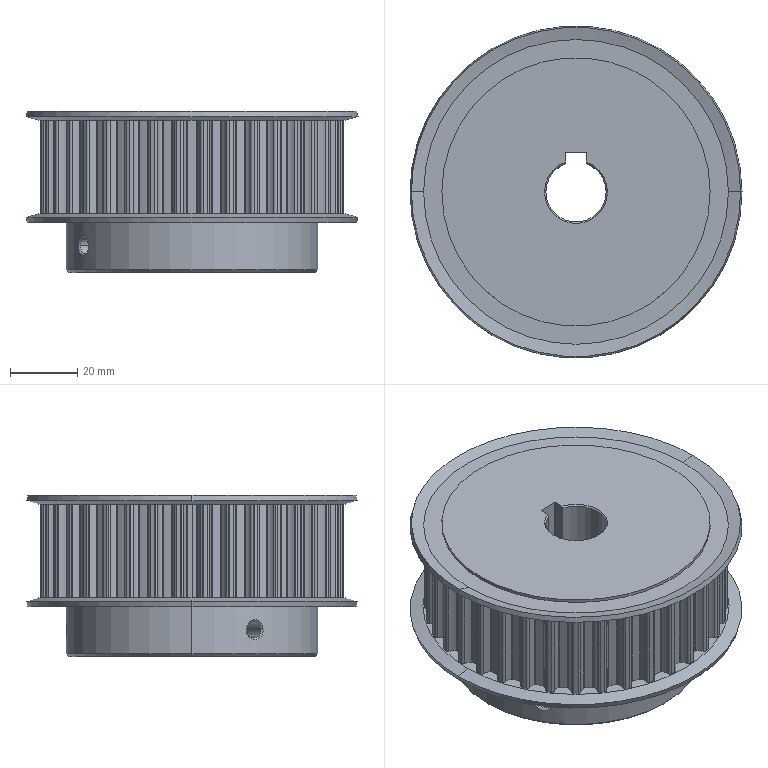Part | SolidWorks | features BaseBody 1 | 1 solid | 370 faces | box 99 x 99 x 48.077 mm | volume 252335 mm3 | cylinder 336 | cone 24 | plane 10 | commonest cylinder face diameters 1.5 x88 0.8 x84 10.6 x76 84.64 x37 90.3 x36 4.917 x4